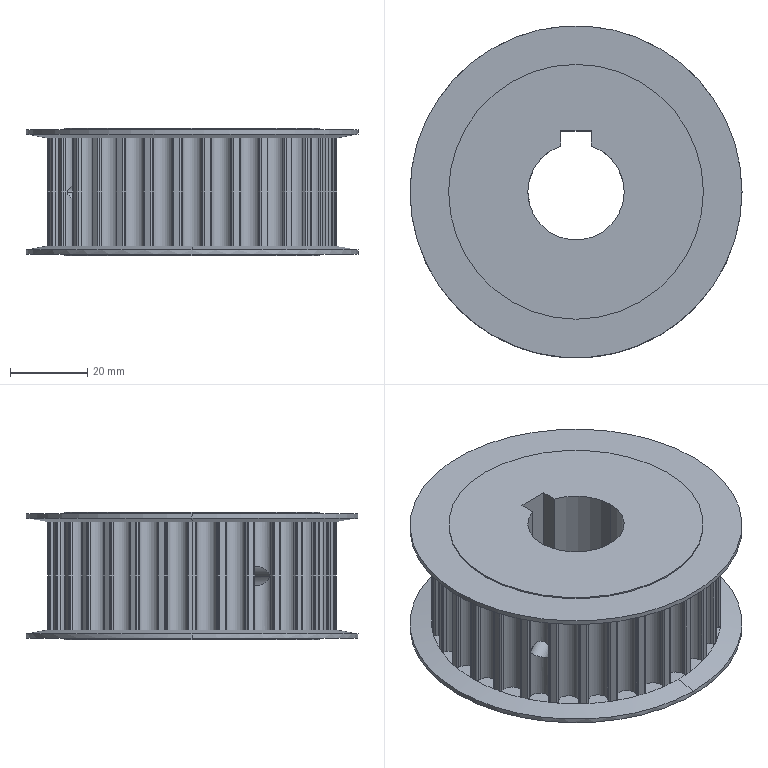Part | SolidWorks | features BaseBody 1 | 1 solid | 295 faces | box 86 x 86 x 33 mm | volume 118821 mm3 | cylinder 164 | plane 127 | cone 4 | commonest cylinder face diameters 0.81 x74 5.199 x44 75.02 x31 5 x4 66 x4 86 x4